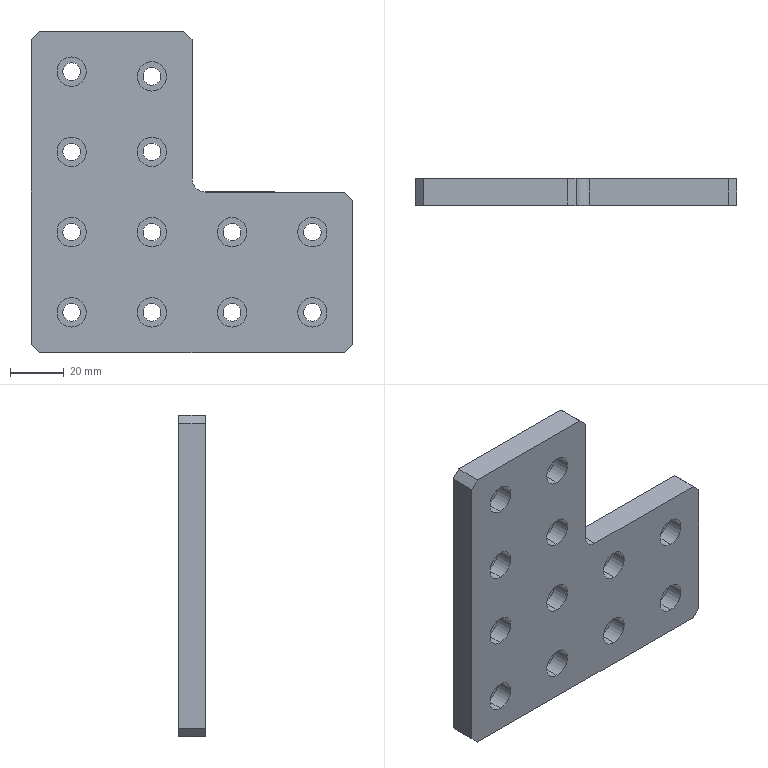Part | SolidWorks | features Chamfer 1, Extrusion 1, Fillet 1, HoleWzd 1, ICE 1 | 1 solid | 74 faces | box 120 x 10 x 120 mm | volume 98760 mm3 | cylinder 49 | plane 25 | commonest cylinder face diameters 6.6 x24 11 x24 10 x1